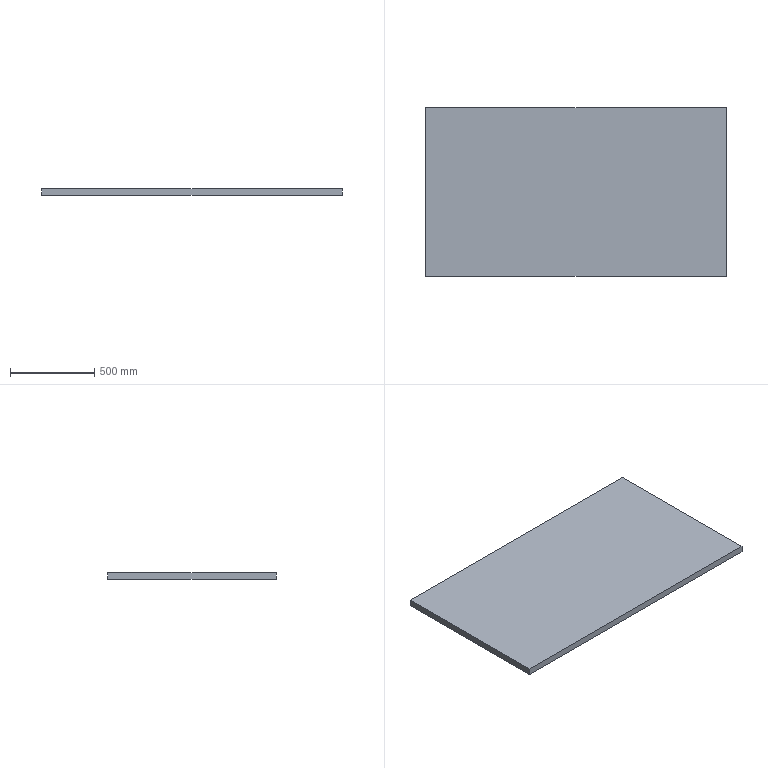Part | SolidWorks | features Extrusion 1 | 1 solid | 6 faces | box 1780 x 1000 x 40 mm | volume 71200000 mm3 | plane 6
STEP:
#1=CARTESIAN_POINT('',(1780.,0.,0.));
#2=VERTEX_POINT('',#1);
#3=CARTESIAN_POINT('',(1780.,1000.,0.));
#4=VERTEX_POINT('',#3);
#5=CARTESIAN_POINT('',(1780.,500.,0.));
#6=DIRECTION('',(0.,1.,0.));
#7=VECTOR('',#6,1000.);
#8=LINE('',#5,#7);
#9=EDGE_CURVE('',#2,#4,#8,.T.);
#10=ORIENTED_EDGE('',*,*,#9,.T.);
#11=CARTESIAN_POINT('',(1780.,1000.,40.));
#12=VERTEX_POINT('',#11);
#13=CARTESIAN_POINT('',(1780.,1000.,40.));
#14=DIRECTION('',(0.,0.,-1.));
#15=VECTOR('',#14,1000.);
#16=LINE('',#13,#15);
#17=EDGE_CURVE('',#12,#4,#16,.T.);
#18=ORIENTED_EDGE('',*,*,#17,.F.);
#19=CARTESIAN_POINT('',(1780.,0.,40.));
#20=VERTEX_POINT('',#19);
#21=CARTESIAN_POINT('',(1780.,500.,40.));
#22=DIRECTION('',(0.,1.,0.));
#23=VECTOR('',#22,1000.);
#24=LINE('',#21,#23);
#25=EDGE_CURVE('',#20,#12,#24,.T.);
#26=ORIENTED_EDGE('',*,*,#25,.F.);
#27=CARTESIAN_POINT('',(1780.,0.,40.));
#28=DIRECTION('',(0.,0.,-1.));
#29=VECTOR('',#28,1000.);
#30=LINE('',#27,#29);
#31=EDGE_CURVE('',#20,#2,#30,.T.);
#32=ORIENTED_EDGE('',*,*,#31,.T.);
#33=EDGE_LOOP('',(#10,#18,#26,#32));
#34=FACE_OUTER_BOUND('',#33,.T.);
#35=CARTESIAN_POINT('',(1780.,500.,40.));
#36=DIRECTION('',(-1.,0.,0.));
#37=DIRECTION('',(0.,0.,1.));
#38=AXIS2_PLACEMENT_3D('',#35,#36,#37);
#39=PLANE('',#38);
#40=ADVANCED_FACE('',(#34),#39,.F.);
#41=CARTESIAN_POINT('',(0.,1000.,0.));
#42=VERTEX_POINT('',#41);
#43=CARTESIAN_POINT('',(0.,1000.,0.));
#44=DIRECTION('',(-1.,0.,0.));
#45=VECTOR('',#44,1000.);
#46=LINE('',#43,#45);
#47=EDGE_CURVE('',#4,#42,#46,.T.);
#48=ORIENTED_EDGE('',*,*,#47,.T.);
#49=CARTESIAN_POINT('',(0.,1000.,40.));
#50=VERTEX_POINT('',#49);
#51=CARTESIAN_POINT('',(0.,1000.,40.));
#52=DIRECTION('',(0.,0.,-1.));
#53=VECTOR('',#52,1000.);
#54=LINE('',#51,#53);
#55=EDGE_CURVE('',#50,#42,#54,.T.);
#56=ORIENTED_EDGE('',*,*,#55,.F.);
#57=CARTESIAN_POINT('',(0.,1000.,40.));
#58=DIRECTION('',(-1.,0.,0.));
#59=VECTOR('',#58,1000.);
#60=LINE('',#57,#59);
#61=EDGE_CURVE('',#12,#50,#60,.T.);
#62=ORIENTED_EDGE('',*,*,#61,.F.);
#63=ORIENTED_EDGE('',*,*,#17,.T.);
#64=EDGE_LOOP('',(#48,#56,#62,#63));
#65=FACE_OUTER_BOUND('',#64,.T.);
#66=CARTESIAN_POINT('',(0.,1000.,40.));
#67=DIRECTION('',(0.,-1.,0.));
#68=DIRECTION('',(0.,0.,-1.));
#69=AXIS2_PLACEMENT_3D('',#66,#67,#68);
#70=PLANE('',#69);
#71=ADVANCED_FACE('',(#65),#70,.F.);
#72=CARTESIAN_POINT('',(0.,0.,0.));
#73=VERTEX_POINT('',#72);
#74=CARTESIAN_POINT('',(0.,0.,0.));
#75=DIRECTION('',(0.,-1.,0.));
#76=VECTOR('',#75,1000.);
#77=LINE('',#74,#76);
#78=EDGE_CURVE('',#42,#73,#77,.T.);
#79=ORIENTED_EDGE('',*,*,#78,.T.);
#80=CARTESIAN_POINT('',(0.,0.,40.));
#81=VERTEX_POINT('',#80);
#82=CARTESIAN_POINT('',(0.,0.,40.));
#83=DIRECTION('',(0.,0.,-1.));
#84=VECTOR('',#83,1000.);
#85=LINE('',#82,#84);
#86=EDGE_CURVE('',#81,#73,#85,.T.);
#87=ORIENTED_EDGE('',*,*,#86,.F.);
#88=CARTESIAN_POINT('',(0.,0.,40.));
#89=DIRECTION('',(0.,-1.,0.));
#90=VECTOR('',#89,1000.);
#91=LINE('',#88,#90);
#92=EDGE_CURVE('',#50,#81,#91,.T.);
#93=ORIENTED_EDGE('',*,*,#92,.F.);
#94=ORIENTED_EDGE('',*,*,#55,.T.);
#95=EDGE_LOOP('',(#79,#87,#93,#94));
#96=FACE_OUTER_BOUND('',#95,.T.);
#97=CARTESIAN_POINT('',(0.,0.,40.));
#98=DIRECTION('',(1.,0.,0.));
#99=DIRECTION('',(0.,0.,-1.));
#100=AXIS2_PLACEMENT_3D('',#97,#98,#99);
#101=PLANE('',#100);
#102=ADVANCED_FACE('',(#96),#101,.F.);
#103=CARTESIAN_POINT('',(0.,0.,0.));
#104=DIRECTION('',(1.,0.,0.));
#105=VECTOR('',#104,1000.);
#106=LINE('',#103,#105);
#107=EDGE_CURVE('',#73,#2,#106,.T.);
#108=ORIENTED_EDGE('',*,*,#107,.T.);
#109=ORIENTED_EDGE('',*,*,#31,.F.);
#110=CARTESIAN_POINT('',(0.,0.,40.));
#111=DIRECTION('',(1.,0.,0.));
#112=VECTOR('',#111,1000.);
#113=LINE('',#110,#112);
#114=EDGE_CURVE('',#81,#20,#113,.T.);
#115=ORIENTED_EDGE('',*,*,#114,.F.);
#116=ORIENTED_EDGE('',*,*,#86,.T.);
#117=EDGE_LOOP('',(#108,#109,#115,#116));
#118=FACE_OUTER_BOUND('',#117,.T.);
#119=CARTESIAN_POINT('',(0.,0.,40.));
#120=DIRECTION('',(0.,1.,0.));
#121=DIRECTION('',(0.,0.,1.));
#122=AXIS2_PLACEMENT_3D('',#119,#120,#121);
#123=PLANE('',#122);
#124=ADVANCED_FACE('',(#118),#123,.F.);
#125=ORIENTED_EDGE('',*,*,#25,.T.);
#126=ORIENTED_EDGE('',*,*,#61,.T.);
#127=ORIENTED_EDGE('',*,*,#92,.T.);
#128=ORIENTED_EDGE('',*,*,#114,.T.);
#129=EDGE_LOOP('',(#125,#126,#127,#128));
#130=FACE_OUTER_BOUND('',#129,.T.);
#131=CARTESIAN_POINT('',(0.,0.,40.));
#132=DIRECTION('',(0.,0.,1.));
#133=DIRECTION('',(1.,0.,0.));
#134=AXIS2_PLACEMENT_3D('',#131,#132,#133);
#135=PLANE('',#134);
#136=ADVANCED_FACE('',(#130),#135,.T.);
#137=ORIENTED_EDGE('',*,*,#9,.F.);
#138=ORIENTED_EDGE('',*,*,#107,.F.);
#139=ORIENTED_EDGE('',*,*,#78,.F.);
#140=ORIENTED_EDGE('',*,*,#47,.F.);
#141=EDGE_LOOP('',(#137,#138,#139,#140));
#142=FACE_OUTER_BOUND('',#141,.T.);
#143=CARTESIAN_POINT('',(0.,0.,0.));
#144=DIRECTION('',(0.,0.,1.));
#145=DIRECTION('',(1.,0.,0.));
#146=AXIS2_PLACEMENT_3D('',#143,#144,#145);
#147=PLANE('',#146);
#148=ADVANCED_FACE('',(#142),#147,.F.);
#149=CLOSED_SHELL('',(#40,#71,#102,#124,#136,#148));
#150=MANIFOLD_SOLID_BREP('',#149);
#151=CARTESIAN_POINT('',(0.,0.,0.));
#152=DIRECTION('',(0.,0.,1.));
#153=DIRECTION('',(1.,0.,0.));
#154=AXIS2_PLACEMENT_3D('',#151,#152,#153);
#155=(LENGTH_UNIT()NAMED_UNIT(*)SI_UNIT(.MILLI.,.METRE.));
#156=UNCERTAINTY_MEASURE_WITH_UNIT(LENGTH_MEASURE(0.00001),#155,'','');
#157=(NAMED_UNIT(*)PLANE_ANGLE_UNIT()SI_UNIT($,.RADIAN.));
#158=(NAMED_UNIT(*)SI_UNIT($,.STERADIAN.)SOLID_ANGLE_UNIT());
#159=(GEOMETRIC_REPRESENTATION_CONTEXT(3)GLOBAL_UNCERTAINTY_ASSIGNED_CONTEXT((#156))GLOBAL_UNIT_ASSIGNED_CONTEXT((#155,#157,#158))REPRESENTATION_CONTEXT('',''));
#160=ADVANCED_BREP_SHAPE_REPRESENTATION('',(#150,#154),#159);